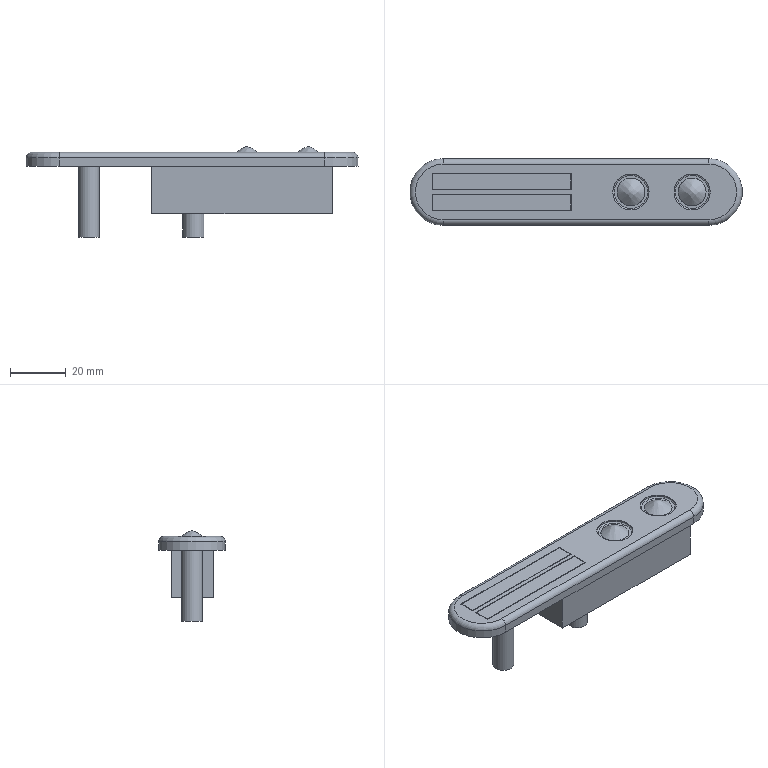Part | STEP file | Q7C1216W | 1 solid | 71 faces | box 119.5 x 24 x 32.509 mm | volume 28513 mm3 | plane 41 | cylinder 24 | torus 4 | spline 2 | commonest cylinder face diameters 0.4 x8 3.5 x3 7.5 x3 4 x2 10 x2 13 x2